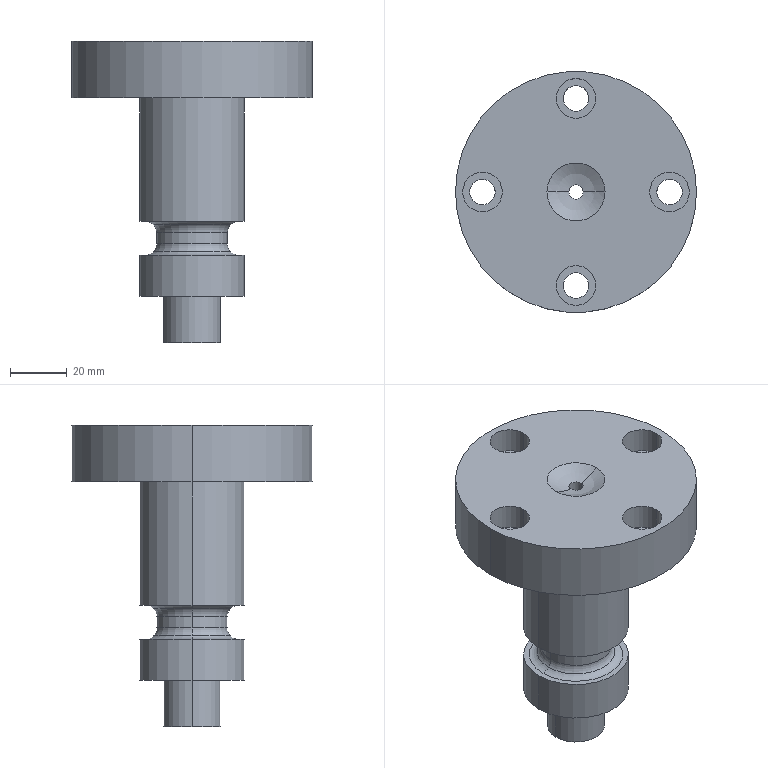Part | Creo | 1 solid | 48 faces | box 85 x 85 x 106.339 mm | volume 174751 mm3 | cylinder 26 | plane 10 | torus 8 | sphere 2 | cone 2 | commonest cylinder face diameters 9 x8 14 x8 37 x4 20 x2 25 x2 85 x2
STEP:
#1=CARTESIAN_POINT('',(18.5,0.,127.5));
#2=VERTEX_POINT('',#1);
#3=CARTESIAN_POINT('',(-18.5,0.,127.5));
#4=VERTEX_POINT('',#3);
#5=CARTESIAN_POINT('',(0.,0.,127.5));
#6=DIRECTION('',(0.,0.,1.));
#7=DIRECTION('',(1.,0.,0.));
#8=AXIS2_PLACEMENT_3D('',#5,#6,#7);
#9=CIRCLE('',#8,18.5);
#10=EDGE_CURVE('',#2,#4,#9,.T.);
#11=ORIENTED_EDGE('',*,*,#10,.T.);
#12=CARTESIAN_POINT('',(-18.5,0.,84.));
#13=VERTEX_POINT('',#12);
#14=CARTESIAN_POINT('',(-18.5,0.,127.5));
#15=DIRECTION('',(0.,0.,-1.));
#16=VECTOR('',#15,43.5);
#17=LINE('',#14,#16);
#18=EDGE_CURVE('',#4,#13,#17,.T.);
#19=ORIENTED_EDGE('',*,*,#18,.T.);
#20=CARTESIAN_POINT('',(18.5,0.,84.));
#21=VERTEX_POINT('',#20);
#22=CARTESIAN_POINT('',(0.,0.,84.));
#23=DIRECTION('',(0.,0.,-1.));
#24=DIRECTION('',(-1.,0.,0.));
#25=AXIS2_PLACEMENT_3D('',#22,#23,#24);
#26=CIRCLE('',#25,18.5);
#27=EDGE_CURVE('',#13,#21,#26,.T.);
#28=ORIENTED_EDGE('',*,*,#27,.T.);
#29=CARTESIAN_POINT('',(18.5,0.,127.5));
#30=DIRECTION('',(0.,0.,-1.));
#31=VECTOR('',#30,43.5);
#32=LINE('',#29,#31);
#33=EDGE_CURVE('',#2,#21,#32,.T.);
#34=ORIENTED_EDGE('',*,*,#33,.F.);
#35=EDGE_LOOP('',(#11,#19,#28,#34));
#36=FACE_OUTER_BOUND('',#35,.F.);
#37=CARTESIAN_POINT('',(0.,0.,127.5));
#38=DIRECTION('',(0.,0.,-1.));
#39=DIRECTION('',(-1.,0.,0.));
#40=AXIS2_PLACEMENT_3D('',#37,#38,#39);
#41=CYLINDRICAL_SURFACE('',#40,18.5);
#42=ADVANCED_FACE('',(#36),#41,.T.);
#43=CARTESIAN_POINT('',(42.5,0.,127.5));
#44=VERTEX_POINT('',#43);
#45=CARTESIAN_POINT('',(-42.5,0.,127.5));
#46=VERTEX_POINT('',#45);
#47=CARTESIAN_POINT('',(0.,0.,127.5));
#48=DIRECTION('',(0.,0.,-1.));
#49=DIRECTION('',(1.,0.,0.));
#50=AXIS2_PLACEMENT_3D('',#47,#48,#49);
#51=CIRCLE('',#50,42.5);
#52=EDGE_CURVE('',#44,#46,#51,.T.);
#53=ORIENTED_EDGE('',*,*,#52,.F.);
#54=CARTESIAN_POINT('',(0.,0.,127.5));
#55=DIRECTION('',(0.,0.,-1.));
#56=DIRECTION('',(-1.,0.,0.));
#57=AXIS2_PLACEMENT_3D('',#54,#55,#56);
#58=CIRCLE('',#57,42.5);
#59=EDGE_CURVE('',#46,#44,#58,.T.);
#60=ORIENTED_EDGE('',*,*,#59,.F.);
#61=EDGE_LOOP('',(#53,#60));
#62=FACE_OUTER_BOUND('',#61,.F.);
#63=CARTESIAN_POINT('',(-28.5,0.,127.5));
#64=VERTEX_POINT('',#63);
#65=CARTESIAN_POINT('',(-37.5,0.,127.5));
#66=VERTEX_POINT('',#65);
#67=CARTESIAN_POINT('',(-33.,0.,127.5));
#68=DIRECTION('',(0.,0.,1.));
#69=DIRECTION('',(1.,0.,0.));
#70=AXIS2_PLACEMENT_3D('',#67,#68,#69);
#71=CIRCLE('',#70,4.5);
#72=EDGE_CURVE('',#64,#66,#71,.T.);
#73=ORIENTED_EDGE('',*,*,#72,.F.);
#74=CARTESIAN_POINT('',(-33.,0.,127.5));
#75=DIRECTION('',(0.,0.,1.));
#76=DIRECTION('',(-1.,0.,0.));
#77=AXIS2_PLACEMENT_3D('',#74,#75,#76);
#78=CIRCLE('',#77,4.5);
#79=EDGE_CURVE('',#66,#64,#78,.T.);
#80=ORIENTED_EDGE('',*,*,#79,.F.);
#81=EDGE_LOOP('',(#73,#80));
#82=FACE_BOUND('',#81,.F.);
#83=CARTESIAN_POINT('',(0.,0.,127.5));
#84=DIRECTION('',(0.,0.,1.));
#85=DIRECTION('',(-1.,0.,0.));
#86=AXIS2_PLACEMENT_3D('',#83,#84,#85);
#87=CIRCLE('',#86,18.5);
#88=EDGE_CURVE('',#4,#2,#87,.T.);
#89=ORIENTED_EDGE('',*,*,#88,.F.);
#90=ORIENTED_EDGE('',*,*,#10,.F.);
#91=EDGE_LOOP('',(#89,#90));
#92=FACE_BOUND('',#91,.F.);
#93=CARTESIAN_POINT('',(4.5,33.,127.5));
#94=VERTEX_POINT('',#93);
#95=CARTESIAN_POINT('',(-4.5,33.,127.5));
#96=VERTEX_POINT('',#95);
#97=CARTESIAN_POINT('',(0.,33.,127.5));
#98=DIRECTION('',(0.,0.,1.));
#99=DIRECTION('',(1.,0.,0.));
#100=AXIS2_PLACEMENT_3D('',#97,#98,#99);
#101=CIRCLE('',#100,4.5);
#102=EDGE_CURVE('',#94,#96,#101,.T.);
#103=ORIENTED_EDGE('',*,*,#102,.F.);
#104=CARTESIAN_POINT('',(0.,33.,127.5));
#105=DIRECTION('',(0.,0.,1.));
#106=DIRECTION('',(-1.,0.,0.));
#107=AXIS2_PLACEMENT_3D('',#104,#105,#106);
#108=CIRCLE('',#107,4.5);
#109=EDGE_CURVE('',#96,#94,#108,.T.);
#110=ORIENTED_EDGE('',*,*,#109,.F.);
#111=EDGE_LOOP('',(#103,#110));
#112=FACE_BOUND('',#111,.F.);
#113=CARTESIAN_POINT('',(4.5,-33.,127.5));
#114=VERTEX_POINT('',#113);
#115=CARTESIAN_POINT('',(-4.5,-33.,127.5));
#116=VERTEX_POINT('',#115);
#117=CARTESIAN_POINT('',(0.,-33.,127.5));
#118=DIRECTION('',(0.,0.,1.));
#119=DIRECTION('',(1.,0.,0.));
#120=AXIS2_PLACEMENT_3D('',#117,#118,#119);
#121=CIRCLE('',#120,4.5);
#122=EDGE_CURVE('',#114,#116,#121,.T.);
#123=ORIENTED_EDGE('',*,*,#122,.F.);
#124=CARTESIAN_POINT('',(0.,-33.,127.5));
#125=DIRECTION('',(0.,0.,1.));
#126=DIRECTION('',(-1.,0.,0.));
#127=AXIS2_PLACEMENT_3D('',#124,#125,#126);
#128=CIRCLE('',#127,4.5);
#129=EDGE_CURVE('',#116,#114,#128,.T.);
#130=ORIENTED_EDGE('',*,*,#129,.F.);
#131=EDGE_LOOP('',(#123,#130));
#132=FACE_BOUND('',#131,.F.);
#133=CARTESIAN_POINT('',(37.5,0.,127.5));
#134=VERTEX_POINT('',#133);
#135=CARTESIAN_POINT('',(28.5,0.,127.5));
#136=VERTEX_POINT('',#135);
#137=CARTESIAN_POINT('',(33.,0.,127.5));
#138=DIRECTION('',(0.,0.,1.));
#139=DIRECTION('',(1.,0.,0.));
#140=AXIS2_PLACEMENT_3D('',#137,#138,#139);
#141=CIRCLE('',#140,4.5);
#142=EDGE_CURVE('',#134,#136,#141,.T.);
#143=ORIENTED_EDGE('',*,*,#142,.F.);
#144=CARTESIAN_POINT('',(33.,0.,127.5));
#145=DIRECTION('',(0.,0.,1.));
#146=DIRECTION('',(-1.,0.,0.));
#147=AXIS2_PLACEMENT_3D('',#144,#145,#146);
#148=CIRCLE('',#147,4.5);
#149=EDGE_CURVE('',#136,#134,#148,.T.);
#150=ORIENTED_EDGE('',*,*,#149,.F.);
#151=EDGE_LOOP('',(#143,#150));
#152=FACE_BOUND('',#151,.F.);
#153=CARTESIAN_POINT('',(0.,0.,127.5));
#154=DIRECTION('',(0.,0.,-1.));
#155=DIRECTION('',(-1.,0.,0.));
#156=AXIS2_PLACEMENT_3D('',#153,#154,#155);
#157=PLANE('',#156);
#158=ADVANCED_FACE('',(#62,#82,#92,#112,#132,#152),#157,.T.);
#159=CARTESIAN_POINT('',(-4.5,33.,138.5));
#160=VERTEX_POINT('',#159);
#161=CARTESIAN_POINT('',(4.5,33.,138.5));
#162=VERTEX_POINT('',#161);
#163=CARTESIAN_POINT('',(0.,33.,138.5));
#164=DIRECTION('',(0.,0.,-1.));
#165=DIRECTION('',(-1.,0.,0.));
#166=AXIS2_PLACEMENT_3D('',#163,#164,#165);
#167=CIRCLE('',#166,4.5);
#168=EDGE_CURVE('',#160,#162,#167,.T.);
#169=ORIENTED_EDGE('',*,*,#168,.T.);
#170=CARTESIAN_POINT('',(4.5,33.,127.5));
#171=DIRECTION('',(0.,0.,1.));
#172=VECTOR('',#171,11.);
#173=LINE('',#170,#172);
#174=EDGE_CURVE('',#94,#162,#173,.T.);
#175=ORIENTED_EDGE('',*,*,#174,.F.);
#176=ORIENTED_EDGE('',*,*,#102,.T.);
#177=CARTESIAN_POINT('',(-4.5,33.,127.5));
#178=DIRECTION('',(0.,0.,1.));
#179=VECTOR('',#178,11.);
#180=LINE('',#177,#179);
#181=EDGE_CURVE('',#96,#160,#180,.T.);
#182=ORIENTED_EDGE('',*,*,#181,.T.);
#183=EDGE_LOOP('',(#169,#175,#176,#182));
#184=FACE_OUTER_BOUND('',#183,.F.);
#185=CARTESIAN_POINT('',(0.,33.,127.5));
#186=DIRECTION('',(0.,0.,1.));
#187=DIRECTION('',(1.,0.,0.));
#188=AXIS2_PLACEMENT_3D('',#185,#186,#187);
#189=CYLINDRICAL_SURFACE('',#188,4.5);
#190=ADVANCED_FACE('',(#184),#189,.F.);
#191=CARTESIAN_POINT('',(7.,33.,138.5));
#192=VERTEX_POINT('',#191);
#193=CARTESIAN_POINT('',(-7.,33.,138.5));
#194=VERTEX_POINT('',#193);
#195=CARTESIAN_POINT('',(0.,33.,138.5));
#196=DIRECTION('',(0.,0.,1.));
#197=DIRECTION('',(1.,0.,0.));
#198=AXIS2_PLACEMENT_3D('',#195,#196,#197);
#199=CIRCLE('',#198,7.);
#200=EDGE_CURVE('',#192,#194,#199,.T.);
#201=ORIENTED_EDGE('',*,*,#200,.F.);
#202=CARTESIAN_POINT('',(0.,33.,138.5));
#203=DIRECTION('',(0.,0.,1.));
#204=DIRECTION('',(-1.,0.,0.));
#205=AXIS2_PLACEMENT_3D('',#202,#203,#204);
#206=CIRCLE('',#205,7.);
#207=EDGE_CURVE('',#194,#192,#206,.T.);
#208=ORIENTED_EDGE('',*,*,#207,.F.);
#209=EDGE_LOOP('',(#201,#208));
#210=FACE_OUTER_BOUND('',#209,.F.);
#211=CARTESIAN_POINT('',(0.,33.,138.5));
#212=DIRECTION('',(0.,0.,-1.));
#213=DIRECTION('',(1.,0.,0.));
#214=AXIS2_PLACEMENT_3D('',#211,#212,#213);
#215=CIRCLE('',#214,4.5);
#216=EDGE_CURVE('',#162,#160,#215,.T.);
#217=ORIENTED_EDGE('',*,*,#216,.F.);
#218=ORIENTED_EDGE('',*,*,#168,.F.);
#219=EDGE_LOOP('',(#217,#218));
#220=FACE_BOUND('',#219,.F.);
#221=CARTESIAN_POINT('',(0.,33.,138.5));
#222=DIRECTION('',(0.,0.,-1.));
#223=DIRECTION('',(-1.,0.,0.));
#224=AXIS2_PLACEMENT_3D('',#221,#222,#223);
#225=PLANE('',#224);
#226=ADVANCED_FACE('',(#210,#220),#225,.F.);
#227=ORIENTED_EDGE('',*,*,#216,.T.);
#228=ORIENTED_EDGE('',*,*,#181,.F.);
#229=ORIENTED_EDGE('',*,*,#109,.T.);
#230=ORIENTED_EDGE('',*,*,#174,.T.);
#231=EDGE_LOOP('',(#227,#228,#229,#230));
#232=FACE_OUTER_BOUND('',#231,.F.);
#233=CARTESIAN_POINT('',(0.,33.,127.5));
#234=DIRECTION('',(0.,0.,1.));
#235=DIRECTION('',(1.,0.,0.));
#236=AXIS2_PLACEMENT_3D('',#233,#234,#235);
#237=CYLINDRICAL_SURFACE('',#236,4.5);
#238=ADVANCED_FACE('',(#232),#237,.F.);
#239=CARTESIAN_POINT('',(-7.,33.,147.5));
#240=VERTEX_POINT('',#239);
#241=CARTESIAN_POINT('',(7.,33.,147.5));
#242=VERTEX_POINT('',#241);
#243=CARTESIAN_POINT('',(0.,33.,147.5));
#244=DIRECTION('',(0.,0.,-1.));
#245=DIRECTION('',(-1.,0.,0.));
#246=AXIS2_PLACEMENT_3D('',#243,#244,#245);
#247=CIRCLE('',#246,7.);
#248=EDGE_CURVE('',#240,#242,#247,.T.);
#249=ORIENTED_EDGE('',*,*,#248,.T.);
#250=CARTESIAN_POINT('',(7.,33.,138.5));
#251=DIRECTION('',(0.,0.,1.));
#252=VECTOR('',#251,9.);
#253=LINE('',#250,#252);
#254=EDGE_CURVE('',#192,#242,#253,.T.);
#255=ORIENTED_EDGE('',*,*,#254,.F.);
#256=ORIENTED_EDGE('',*,*,#200,.T.);
#257=CARTESIAN_POINT('',(-7.,33.,138.5));
#258=DIRECTION('',(0.,0.,1.));
#259=VECTOR('',#258,9.);
#260=LINE('',#257,#259);
#261=EDGE_CURVE('',#194,#240,#260,.T.);
#262=ORIENTED_EDGE('',*,*,#261,.T.);
#263=EDGE_LOOP('',(#249,#255,#256,#262));
#264=FACE_OUTER_BOUND('',#263,.F.);
#265=CARTESIAN_POINT('',(0.,33.,138.5));
#266=DIRECTION('',(0.,0.,1.));
#267=DIRECTION('',(1.,0.,0.));
#268=AXIS2_PLACEMENT_3D('',#265,#266,#267);
#269=CYLINDRICAL_SURFACE('',#268,7.);
#270=ADVANCED_FACE('',(#264),#269,.F.);
#271=CARTESIAN_POINT('',(-42.5,0.,147.5));
#272=VERTEX_POINT('',#271);
#273=CARTESIAN_POINT('',(42.5,0.,147.5));
#274=VERTEX_POINT('',#273);
#275=CARTESIAN_POINT('',(0.,0.,147.5));
#276=DIRECTION('',(0.,0.,1.));
#277=DIRECTION('',(-1.,0.,0.));
#278=AXIS2_PLACEMENT_3D('',#275,#276,#277);
#279=CIRCLE('',#278,42.5);
#280=EDGE_CURVE('',#272,#274,#279,.T.);
#281=ORIENTED_EDGE('',*,*,#280,.F.);
#282=CARTESIAN_POINT('',(0.,0.,147.5));
#283=DIRECTION('',(0.,0.,1.));
#284=DIRECTION('',(1.,0.,0.));
#285=AXIS2_PLACEMENT_3D('',#282,#283,#284);
#286=CIRCLE('',#285,42.5);
#287=EDGE_CURVE('',#274,#272,#286,.T.);
#288=ORIENTED_EDGE('',*,*,#287,.F.);
#289=EDGE_LOOP('',(#281,#288));
#290=FACE_OUTER_BOUND('',#289,.F.);
#291=CARTESIAN_POINT('',(0.,33.,147.5));
#292=DIRECTION('',(0.,0.,-1.));
#293=DIRECTION('',(1.,0.,0.));
#294=AXIS2_PLACEMENT_3D('',#291,#292,#293);
#295=CIRCLE('',#294,7.);
#296=EDGE_CURVE('',#242,#240,#295,.T.);
#297=ORIENTED_EDGE('',*,*,#296,.F.);
#298=ORIENTED_EDGE('',*,*,#248,.F.);
#299=EDGE_LOOP('',(#297,#298));
#300=FACE_BOUND('',#299,.F.);
#301=CARTESIAN_POINT('',(7.,-33.,147.5));
#302=VERTEX_POINT('',#301);
#303=CARTESIAN_POINT('',(-7.,-33.,147.5));
#304=VERTEX_POINT('',#303);
#305=CARTESIAN_POINT('',(0.,-33.,147.5));
#306=DIRECTION('',(0.,0.,-1.));
#307=DIRECTION('',(1.,0.,0.));
#308=AXIS2_PLACEMENT_3D('',#305,#306,#307);
#309=CIRCLE('',#308,7.);
#310=EDGE_CURVE('',#302,#304,#309,.T.);
#311=ORIENTED_EDGE('',*,*,#310,.F.);
#312=CARTESIAN_POINT('',(0.,-33.,147.5));
#313=DIRECTION('',(0.,0.,-1.));
#314=DIRECTION('',(-1.,0.,0.));
#315=AXIS2_PLACEMENT_3D('',#312,#313,#314);
#316=CIRCLE('',#315,7.);
#317=EDGE_CURVE('',#304,#302,#316,.T.);
#318=ORIENTED_EDGE('',*,*,#317,.F.);
#319=EDGE_LOOP('',(#311,#318));
#320=FACE_BOUND('',#319,.F.);
#321=CARTESIAN_POINT('',(-26.,0.,147.5));
#322=VERTEX_POINT('',#321);
#323=CARTESIAN_POINT('',(-40.,0.,147.5));
#324=VERTEX_POINT('',#323);
#325=CARTESIAN_POINT('',(-33.,0.,147.5));
#326=DIRECTION('',(0.,0.,-1.));
#327=DIRECTION('',(1.,0.,0.));
#328=AXIS2_PLACEMENT_3D('',#325,#326,#327);
#329=CIRCLE('',#328,7.);
#330=EDGE_CURVE('',#322,#324,#329,.T.);
#331=ORIENTED_EDGE('',*,*,#330,.F.);
#332=CARTESIAN_POINT('',(-33.,0.,147.5));
#333=DIRECTION('',(0.,0.,-1.));
#334=DIRECTION('',(-1.,0.,0.));
#335=AXIS2_PLACEMENT_3D('',#332,#333,#334);
#336=CIRCLE('',#335,7.);
#337=EDGE_CURVE('',#324,#322,#336,.T.);
#338=ORIENTED_EDGE('',*,*,#337,.F.);
#339=EDGE_LOOP('',(#331,#338));
#340=FACE_BOUND('',#339,.F.);
#341=CARTESIAN_POINT('',(10.247,0.,147.5));
#342=VERTEX_POINT('',#341);
#343=CARTESIAN_POINT('',(-10.247,0.,147.5));
#344=VERTEX_POINT('',#343);
#345=CARTESIAN_POINT('',(0.,0.,147.5));
#346=DIRECTION('',(0.,0.,-1.));
#347=DIRECTION('',(1.,0.,0.));
#348=AXIS2_PLACEMENT_3D('',#345,#346,#347);
#349=CIRCLE('',#348,10.247);
#350=EDGE_CURVE('',#342,#344,#349,.T.);
#351=ORIENTED_EDGE('',*,*,#350,.F.);
#352=CARTESIAN_POINT('',(0.,0.,147.5));
#353=DIRECTION('',(0.,0.,-1.));
#354=DIRECTION('',(-1.,0.,0.));
#355=AXIS2_PLACEMENT_3D('',#352,#353,#354);
#356=CIRCLE('',#355,10.247);
#357=EDGE_CURVE('',#344,#342,#356,.T.);
#358=ORIENTED_EDGE('',*,*,#357,.F.);
#359=EDGE_LOOP('',(#351,#358));
#360=FACE_BOUND('',#359,.F.);
#361=CARTESIAN_POINT('',(40.,0.,147.5));
#362=VERTEX_POINT('',#361);
#363=CARTESIAN_POINT('',(26.,0.,147.5));
#364=VERTEX_POINT('',#363);
#365=CARTESIAN_POINT('',(33.,0.,147.5));
#366=DIRECTION('',(0.,0.,-1.));
#367=DIRECTION('',(1.,0.,0.));
#368=AXIS2_PLACEMENT_3D('',#365,#366,#367);
#369=CIRCLE('',#368,7.);
#370=EDGE_CURVE('',#362,#364,#369,.T.);
#371=ORIENTED_EDGE('',*,*,#370,.F.);
#372=CARTESIAN_POINT('',(33.,0.,147.5));
#373=DIRECTION('',(0.,0.,-1.));
#374=DIRECTION('',(-1.,0.,0.));
#375=AXIS2_PLACEMENT_3D('',#372,#373,#374);
#376=CIRCLE('',#375,7.);
#377=EDGE_CURVE('',#364,#362,#376,.T.);
#378=ORIENTED_EDGE('',*,*,#377,.F.);
#379=EDGE_LOOP('',(#371,#378));
#380=FACE_BOUND('',#379,.F.);
#381=CARTESIAN_POINT('',(0.,0.,147.5));
#382=DIRECTION('',(0.,0.,1.));
#383=DIRECTION('',(1.,0.,0.));
#384=AXIS2_PLACEMENT_3D('',#381,#382,#383);
#385=PLANE('',#384);
#386=ADVANCED_FACE('',(#290,#300,#320,#340,#360,#380),#385,.T.);
#387=ORIENTED_EDGE('',*,*,#370,.T.);
#388=CARTESIAN_POINT('',(26.,0.,138.5));
#389=VERTEX_POINT('',#388);
#390=CARTESIAN_POINT('',(26.,0.,138.5));
#391=DIRECTION('',(0.,0.,1.));
#392=VECTOR('',#391,9.);
#393=LINE('',#390,#392);
#394=EDGE_CURVE('',#389,#364,#393,.T.);
#395=ORIENTED_EDGE('',*,*,#394,.F.);
#396=CARTESIAN_POINT('',(40.,0.,138.5));
#397=VERTEX_POINT('',#396);
#398=CARTESIAN_POINT('',(33.,0.,138.5));
#399=DIRECTION('',(0.,0.,1.));
#400=DIRECTION('',(-1.,0.,0.));
#401=AXIS2_PLACEMENT_3D('',#398,#399,#400);
#402=CIRCLE('',#401,7.);
#403=EDGE_CURVE('',#389,#397,#402,.T.);
#404=ORIENTED_EDGE('',*,*,#403,.T.);
#405=CARTESIAN_POINT('',(40.,0.,138.5));
#406=DIRECTION('',(0.,0.,1.));
#407=VECTOR('',#406,9.);
#408=LINE('',#405,#407);
#409=EDGE_CURVE('',#397,#362,#408,.T.);
#410=ORIENTED_EDGE('',*,*,#409,.T.);
#411=EDGE_LOOP('',(#387,#395,#404,#410));
#412=FACE_OUTER_BOUND('',#411,.F.);
#413=CARTESIAN_POINT('',(33.,0.,138.5));
#414=DIRECTION('',(0.,0.,1.));
#415=DIRECTION('',(1.,0.,0.));
#416=AXIS2_PLACEMENT_3D('',#413,#414,#415);
#417=CYLINDRICAL_SURFACE('',#416,7.);
#418=ADVANCED_FACE('',(#412),#417,.F.);
#419=ORIENTED_EDGE('',*,*,#377,.T.);
#420=ORIENTED_EDGE('',*,*,#409,.F.);
#421=CARTESIAN_POINT('',(33.,0.,138.5));
#422=DIRECTION('',(0.,0.,1.));
#423=DIRECTION('',(1.,0.,0.));
#424=AXIS2_PLACEMENT_3D('',#421,#422,#423);
#425=CIRCLE('',#424,7.);
#426=EDGE_CURVE('',#397,#389,#425,.T.);
#427=ORIENTED_EDGE('',*,*,#426,.T.);
#428=ORIENTED_EDGE('',*,*,#394,.T.);
#429=EDGE_LOOP('',(#419,#420,#427,#428));
#430=FACE_OUTER_BOUND('',#429,.F.);
#431=CARTESIAN_POINT('',(33.,0.,138.5));
#432=DIRECTION('',(0.,0.,1.));
#433=DIRECTION('',(1.,0.,0.));
#434=AXIS2_PLACEMENT_3D('',#431,#432,#433);
#435=CYLINDRICAL_SURFACE('',#434,7.);
#436=ADVANCED_FACE('',(#430),#435,.F.);
#437=ORIENTED_EDGE('',*,*,#426,.F.);
#438=ORIENTED_EDGE('',*,*,#403,.F.);
#439=EDGE_LOOP('',(#437,#438));
#440=FACE_OUTER_BOUND('',#439,.F.);
#441=CARTESIAN_POINT('',(37.5,0.,138.5));
#442=VERTEX_POINT('',#441);
#443=CARTESIAN_POINT('',(28.5,0.,138.5));
#444=VERTEX_POINT('',#443);
#445=CARTESIAN_POINT('',(33.,0.,138.5));
#446=DIRECTION('',(0.,0.,-1.));
#447=DIRECTION('',(1.,0.,0.));
#448=AXIS2_PLACEMENT_3D('',#445,#446,#447);
#449=CIRCLE('',#448,4.5);
#450=EDGE_CURVE('',#442,#444,#449,.T.);
#451=ORIENTED_EDGE('',*,*,#450,.F.);
#452=CARTESIAN_POINT('',(33.,0.,138.5));
#453=DIRECTION('',(0.,0.,-1.));
#454=DIRECTION('',(-1.,0.,0.));
#455=AXIS2_PLACEMENT_3D('',#452,#453,#454);
#456=CIRCLE('',#455,4.5);
#457=EDGE_CURVE('',#444,#442,#456,.T.);
#458=ORIENTED_EDGE('',*,*,#457,.F.);
#459=EDGE_LOOP('',(#451,#458));
#460=FACE_BOUND('',#459,.F.);
#461=CARTESIAN_POINT('',(33.,0.,138.5));
#462=DIRECTION('',(0.,0.,-1.));
#463=DIRECTION('',(-1.,0.,0.));
#464=AXIS2_PLACEMENT_3D('',#461,#462,#463);
#465=PLANE('',#464);
#466=ADVANCED_FACE('',(#440,#460),#465,.F.);
#467=ORIENTED_EDGE('',*,*,#450,.T.);
#468=CARTESIAN_POINT('',(28.5,0.,127.5));
#469=DIRECTION('',(0.,0.,1.));
#470=VECTOR('',#469,11.);
#471=LINE('',#468,#470);
#472=EDGE_CURVE('',#136,#444,#471,.T.);
#473=ORIENTED_EDGE('',*,*,#472,.F.);
#474=ORIENTED_EDGE('',*,*,#149,.T.);
#475=CARTESIAN_POINT('',(37.5,0.,127.5));
#476=DIRECTION('',(0.,0.,1.));
#477=VECTOR('',#476,11.);
#478=LINE('',#475,#477);
#479=EDGE_CURVE('',#134,#442,#478,.T.);
#480=ORIENTED_EDGE('',*,*,#479,.T.);
#481=EDGE_LOOP('',(#467,#473,#474,#480));
#482=FACE_OUTER_BOUND('',#481,.F.);
#483=CARTESIAN_POINT('',(33.,0.,127.5));
#484=DIRECTION('',(0.,0.,1.));
#485=DIRECTION('',(1.,0.,0.));
#486=AXIS2_PLACEMENT_3D('',#483,#484,#485);
#487=CYLINDRICAL_SURFACE('',#486,4.5);
#488=ADVANCED_FACE('',(#482),#487,.F.);
#489=ORIENTED_EDGE('',*,*,#457,.T.);
#490=ORIENTED_EDGE('',*,*,#479,.F.);
#491=ORIENTED_EDGE('',*,*,#142,.T.);
#492=ORIENTED_EDGE('',*,*,#472,.T.);
#493=EDGE_LOOP('',(#489,#490,#491,#492));
#494=FACE_OUTER_BOUND('',#493,.F.);
#495=CARTESIAN_POINT('',(33.,0.,127.5));
#496=DIRECTION('',(0.,0.,1.));
#497=DIRECTION('',(1.,0.,0.));
#498=AXIS2_PLACEMENT_3D('',#495,#496,#497);
#499=CYLINDRICAL_SURFACE('',#498,4.5);
#500=ADVANCED_FACE('',(#494),#499,.F.);
#501=ORIENTED_EDGE('',*,*,#296,.T.);
#502=ORIENTED_EDGE('',*,*,#261,.F.);
#503=ORIENTED_EDGE('',*,*,#207,.T.);
#504=ORIENTED_EDGE('',*,*,#254,.T.);
#505=EDGE_LOOP('',(#501,#502,#503,#504));
#506=FACE_OUTER_BOUND('',#505,.F.);
#507=CARTESIAN_POINT('',(0.,33.,138.5));
#508=DIRECTION('',(0.,0.,1.));
#509=DIRECTION('',(1.,0.,0.));
#510=AXIS2_PLACEMENT_3D('',#507,#508,#509);
#511=CYLINDRICAL_SURFACE('',#510,7.);
#512=ADVANCED_FACE('',(#506),#511,.F.);
#513=ORIENTED_EDGE('',*,*,#310,.T.);
#514=CARTESIAN_POINT('',(-7.,-33.,138.5));
#515=VERTEX_POINT('',#514);
#516=CARTESIAN_POINT('',(-7.,-33.,138.5));
#517=DIRECTION('',(0.,0.,1.));
#518=VECTOR('',#517,9.);
#519=LINE('',#516,#518);
#520=EDGE_CURVE('',#515,#304,#519,.T.);
#521=ORIENTED_EDGE('',*,*,#520,.F.);
#522=CARTESIAN_POINT('',(7.,-33.,138.5));
#523=VERTEX_POINT('',#522);
#524=CARTESIAN_POINT('',(0.,-33.,138.5));
#525=DIRECTION('',(0.,0.,1.));
#526=DIRECTION('',(-1.,0.,0.));
#527=AXIS2_PLACEMENT_3D('',#524,#525,#526);
#528=CIRCLE('',#527,7.);
#529=EDGE_CURVE('',#515,#523,#528,.T.);
#530=ORIENTED_EDGE('',*,*,#529,.T.);
#531=CARTESIAN_POINT('',(7.,-33.,138.5));
#532=DIRECTION('',(0.,0.,1.));
#533=VECTOR('',#532,9.);
#534=LINE('',#531,#533);
#535=EDGE_CURVE('',#523,#302,#534,.T.);
#536=ORIENTED_EDGE('',*,*,#535,.T.);
#537=EDGE_LOOP('',(#513,#521,#530,#536));
#538=FACE_OUTER_BOUND('',#537,.F.);
#539=CARTESIAN_POINT('',(0.,-33.,138.5));
#540=DIRECTION('',(0.,0.,1.));
#541=DIRECTION('',(1.,0.,0.));
#542=AXIS2_PLACEMENT_3D('',#539,#540,#541);
#543=CYLINDRICAL_SURFACE('',#542,7.);
#544=ADVANCED_FACE('',(#538),#543,.F.);
#545=ORIENTED_EDGE('',*,*,#317,.T.);
#546=ORIENTED_EDGE('',*,*,#535,.F.);
#547=CARTESIAN_POINT('',(0.,-33.,138.5));
#548=DIRECTION('',(0.,0.,1.));
#549=DIRECTION('',(1.,0.,0.));
#550=AXIS2_PLACEMENT_3D('',#547,#548,#549);
#551=CIRCLE('',#550,7.);
#552=EDGE_CURVE('',#523,#515,#551,.T.);
#553=ORIENTED_EDGE('',*,*,#552,.T.);
#554=ORIENTED_EDGE('',*,*,#520,.T.);
#555=EDGE_LOOP('',(#545,#546,#553,#554));
#556=FACE_OUTER_BOUND('',#555,.F.);
#557=CARTESIAN_POINT('',(0.,-33.,138.5));
#558=DIRECTION('',(0.,0.,1.));
#559=DIRECTION('',(1.,0.,0.));
#560=AXIS2_PLACEMENT_3D('',#557,#558,#559);
#561=CYLINDRICAL_SURFACE('',#560,7.);
#562=ADVANCED_FACE('',(#556),#561,.F.);
#563=ORIENTED_EDGE('',*,*,#552,.F.);
#564=ORIENTED_EDGE('',*,*,#529,.F.);
#565=EDGE_LOOP('',(#563,#564));
#566=FACE_OUTER_BOUND('',#565,.F.);
#567=CARTESIAN_POINT('',(4.5,-33.,138.5));
#568=VERTEX_POINT('',#567);
#569=CARTESIAN_POINT('',(-4.5,-33.,138.5));
#570=VERTEX_POINT('',#569);
#571=CARTESIAN_POINT('',(0.,-33.,138.5));
#572=DIRECTION('',(0.,0.,-1.));
#573=DIRECTION('',(1.,0.,0.));
#574=AXIS2_PLACEMENT_3D('',#571,#572,#573);
#575=CIRCLE('',#574,4.5);
#576=EDGE_CURVE('',#568,#570,#575,.T.);
#577=ORIENTED_EDGE('',*,*,#576,.F.);
#578=CARTESIAN_POINT('',(0.,-33.,138.5));
#579=DIRECTION('',(0.,0.,-1.));
#580=DIRECTION('',(-1.,0.,0.));
#581=AXIS2_PLACEMENT_3D('',#578,#579,#580);
#582=CIRCLE('',#581,4.5);
#583=EDGE_CURVE('',#570,#568,#582,.T.);
#584=ORIENTED_EDGE('',*,*,#583,.F.);
#585=EDGE_LOOP('',(#577,#584));
#586=FACE_BOUND('',#585,.F.);
#587=CARTESIAN_POINT('',(0.,-33.,138.5));
#588=DIRECTION('',(0.,0.,-1.));
#589=DIRECTION('',(-1.,0.,0.));
#590=AXIS2_PLACEMENT_3D('',#587,#588,#589);
#591=PLANE('',#590);
#592=ADVANCED_FACE('',(#566,#586),#591,.F.);
#593=ORIENTED_EDGE('',*,*,#576,.T.);
#594=CARTESIAN_POINT('',(-4.5,-33.,127.5));
#595=DIRECTION('',(0.,0.,1.));
#596=VECTOR('',#595,11.);
#597=LINE('',#594,#596);
#598=EDGE_CURVE('',#116,#570,#597,.T.);
#599=ORIENTED_EDGE('',*,*,#598,.F.);
#600=ORIENTED_EDGE('',*,*,#129,.T.);
#601=CARTESIAN_POINT('',(4.5,-33.,127.5));
#602=DIRECTION('',(0.,0.,1.));
#603=VECTOR('',#602,11.);
#604=LINE('',#601,#603);
#605=EDGE_CURVE('',#114,#568,#604,.T.);
#606=ORIENTED_EDGE('',*,*,#605,.T.);
#607=EDGE_LOOP('',(#593,#599,#600,#606));
#608=FACE_OUTER_BOUND('',#607,.F.);
#609=CARTESIAN_POINT('',(0.,-33.,127.5));
#610=DIRECTION('',(0.,0.,1.));
#611=DIRECTION('',(1.,0.,0.));
#612=AXIS2_PLACEMENT_3D('',#609,#610,#611);
#613=CYLINDRICAL_SURFACE('',#612,4.5);
#614=ADVANCED_FACE('',(#608),#613,.F.);
#615=ORIENTED_EDGE('',*,*,#583,.T.);
#616=ORIENTED_EDGE('',*,*,#605,.F.);
#617=ORIENTED_EDGE('',*,*,#122,.T.);
#618=ORIENTED_EDGE('',*,*,#598,.T.);
#619=EDGE_LOOP('',(#615,#616,#617,#618));
#620=FACE_OUTER_BOUND('',#619,.F.);
#621=CARTESIAN_POINT('',(0.,-33.,127.5));
#622=DIRECTION('',(0.,0.,1.));
#623=DIRECTION('',(1.,0.,0.));
#624=AXIS2_PLACEMENT_3D('',#621,#622,#623);
#625=CYLINDRICAL_SURFACE('',#624,4.5);
#626=ADVANCED_FACE('',(#620),#625,.F.);
#627=ORIENTED_EDGE('',*,*,#330,.T.);
#628=CARTESIAN_POINT('',(-40.,0.,138.5));
#629=VERTEX_POINT('',#628);
#630=CARTESIAN_POINT('',(-40.,0.,138.5));
#631=DIRECTION('',(0.,0.,1.));
#632=VECTOR('',#631,9.);
#633=LINE('',#630,#632);
#634=EDGE_CURVE('',#629,#324,#633,.T.);
#635=ORIENTED_EDGE('',*,*,#634,.F.);
#636=CARTESIAN_POINT('',(-26.,0.,138.5));
#637=VERTEX_POINT('',#636);
#638=CARTESIAN_POINT('',(-33.,0.,138.5));
#639=DIRECTION('',(0.,0.,1.));
#640=DIRECTION('',(-1.,0.,0.));
#641=AXIS2_PLACEMENT_3D('',#638,#639,#640);
#642=CIRCLE('',#641,7.);
#643=EDGE_CURVE('',#629,#637,#642,.T.);
#644=ORIENTED_EDGE('',*,*,#643,.T.);
#645=CARTESIAN_POINT('',(-26.,0.,138.5));
#646=DIRECTION('',(0.,0.,1.));
#647=VECTOR('',#646,9.);
#648=LINE('',#645,#647);
#649=EDGE_CURVE('',#637,#322,#648,.T.);
#650=ORIENTED_EDGE('',*,*,#649,.T.);
#651=EDGE_LOOP('',(#627,#635,#644,#650));
#652=FACE_OUTER_BOUND('',#651,.F.);
#653=CARTESIAN_POINT('',(-33.,0.,138.5));
#654=DIRECTION('',(0.,0.,1.));
#655=DIRECTION('',(1.,0.,0.));
#656=AXIS2_PLACEMENT_3D('',#653,#654,#655);
#657=CYLINDRICAL_SURFACE('',#656,7.);
#658=ADVANCED_FACE('',(#652),#657,.F.);
#659=ORIENTED_EDGE('',*,*,#337,.T.);
#660=ORIENTED_EDGE('',*,*,#649,.F.);
#661=CARTESIAN_POINT('',(-33.,0.,138.5));
#662=DIRECTION('',(0.,0.,1.));
#663=DIRECTION('',(1.,0.,0.));
#664=AXIS2_PLACEMENT_3D('',#661,#662,#663);
#665=CIRCLE('',#664,7.);
#666=EDGE_CURVE('',#637,#629,#665,.T.);
#667=ORIENTED_EDGE('',*,*,#666,.T.);
#668=ORIENTED_EDGE('',*,*,#634,.T.);
#669=EDGE_LOOP('',(#659,#660,#667,#668));
#670=FACE_OUTER_BOUND('',#669,.F.);
#671=CARTESIAN_POINT('',(-33.,0.,138.5));
#672=DIRECTION('',(0.,0.,1.));
#673=DIRECTION('',(1.,0.,0.));
#674=AXIS2_PLACEMENT_3D('',#671,#672,#673);
#675=CYLINDRICAL_SURFACE('',#674,7.);
#676=ADVANCED_FACE('',(#670),#675,.F.);
#677=ORIENTED_EDGE('',*,*,#666,.F.);
#678=ORIENTED_EDGE('',*,*,#643,.F.);
#679=EDGE_LOOP('',(#677,#678));
#680=FACE_OUTER_BOUND('',#679,.F.);
#681=CARTESIAN_POINT('',(-28.5,0.,138.5));
#682=VERTEX_POINT('',#681);
#683=CARTESIAN_POINT('',(-37.5,0.,138.5));
#684=VERTEX_POINT('',#683);
#685=CARTESIAN_POINT('',(-33.,0.,138.5));
#686=DIRECTION('',(0.,0.,-1.));
#687=DIRECTION('',(1.,0.,0.));
#688=AXIS2_PLACEMENT_3D('',#685,#686,#687);
#689=CIRCLE('',#688,4.5);
#690=EDGE_CURVE('',#682,#684,#689,.T.);
#691=ORIENTED_EDGE('',*,*,#690,.F.);
#692=CARTESIAN_POINT('',(-33.,0.,138.5));
#693=DIRECTION('',(0.,0.,-1.));
#694=DIRECTION('',(-1.,0.,0.));
#695=AXIS2_PLACEMENT_3D('',#692,#693,#694);
#696=CIRCLE('',#695,4.5);
#697=EDGE_CURVE('',#684,#682,#696,.T.);
#698=ORIENTED_EDGE('',*,*,#697,.F.);
#699=EDGE_LOOP('',(#691,#698));
#700=FACE_BOUND('',#699,.F.);
#701=CARTESIAN_POINT('',(-33.,0.,138.5));
#702=DIRECTION('',(0.,0.,-1.));
#703=DIRECTION('',(-1.,0.,0.));
#704=AXIS2_PLACEMENT_3D('',#701,#702,#703);
#705=PLANE('',#704);
#706=ADVANCED_FACE('',(#680,#700),#705,.F.);
#707=ORIENTED_EDGE('',*,*,#690,.T.);
#708=CARTESIAN_POINT('',(-37.5,0.,127.5));
#709=DIRECTION('',(0.,0.,1.));
#710=VECTOR('',#709,11.);
#711=LINE('',#708,#710);
#712=EDGE_CURVE('',#66,#684,#711,.T.);
#713=ORIENTED_EDGE('',*,*,#712,.F.);
#714=ORIENTED_EDGE('',*,*,#79,.T.);
#715=CARTESIAN_POINT('',(-28.5,0.,127.5));
#716=DIRECTION('',(0.,0.,1.));
#717=VECTOR('',#716,11.);
#718=LINE('',#715,#717);
#719=EDGE_CURVE('',#64,#682,#718,.T.);
#720=ORIENTED_EDGE('',*,*,#719,.T.);
#721=EDGE_LOOP('',(#707,#713,#714,#720));
#722=FACE_OUTER_BOUND('',#721,.F.);
#723=CARTESIAN_POINT('',(-33.,0.,127.5));
#724=DIRECTION('',(0.,0.,1.));
#725=DIRECTION('',(1.,0.,0.));
#726=AXIS2_PLACEMENT_3D('',#723,#724,#725);
#727=CYLINDRICAL_SURFACE('',#726,4.5);
#728=ADVANCED_FACE('',(#722),#727,.F.);
#729=ORIENTED_EDGE('',*,*,#697,.T.);
#730=ORIENTED_EDGE('',*,*,#719,.F.);
#731=ORIENTED_EDGE('',*,*,#72,.T.);
#732=ORIENTED_EDGE('',*,*,#712,.T.);
#733=EDGE_LOOP('',(#729,#730,#731,#732));
#734=FACE_OUTER_BOUND('',#733,.F.);
#735=CARTESIAN_POINT('',(-33.,0.,127.5));
#736=DIRECTION('',(0.,0.,1.));
#737=DIRECTION('',(1.,0.,0.));
#738=AXIS2_PLACEMENT_3D('',#735,#736,#737);
#739=CYLINDRICAL_SURFACE('',#738,4.5);
#740=ADVANCED_FACE('',(#734),#739,.F.);
#741=CARTESIAN_POINT('',(2.5,0.,144.665));
#742=VERTEX_POINT('',#741);
#743=CARTESIAN_POINT('',(-2.5,0.,144.665));
#744=VERTEX_POINT('',#743);
#745=CARTESIAN_POINT('',(0.,0.,144.665));
#746=DIRECTION('',(0.,0.,-1.));
#747=DIRECTION('',(1.,0.,0.));
#748=AXIS2_PLACEMENT_3D('',#745,#746,#747);
#749=CIRCLE('',#748,2.5);
#750=EDGE_CURVE('',#742,#744,#749,.T.);
#751=ORIENTED_EDGE('',*,*,#750,.F.);
#752=CARTESIAN_POINT('',(0.,0.,163.5));
#753=DIRECTION('',(0.,-1.,0.));
#754=DIRECTION('',(0.1316,0.,-0.9913));
#755=AXIS2_PLACEMENT_3D('',#752,#753,#754);
#756=CIRCLE('',#755,19.);
#757=EDGE_CURVE('',#742,#342,#756,.T.);
#758=ORIENTED_EDGE('',*,*,#757,.T.);
#759=ORIENTED_EDGE('',*,*,#350,.T.);
#760=CARTESIAN_POINT('',(0.,0.,163.5));
#761=DIRECTION('',(0.,1.,0.));
#762=DIRECTION('',(-0.1316,0.,-0.9913));
#763=AXIS2_PLACEMENT_3D('',#760,#761,#762);
#764=CIRCLE('',#763,19.);
#765=EDGE_CURVE('',#744,#344,#764,.T.);
#766=ORIENTED_EDGE('',*,*,#765,.F.);
#767=EDGE_LOOP('',(#751,#758,#759,#766));
#768=FACE_OUTER_BOUND('',#767,.F.);
#769=CARTESIAN_POINT('',(0.,0.,163.5));
#770=DIRECTION('',(0.,0.,1.));
#771=DIRECTION('',(1.,0.,0.));
#772=AXIS2_PLACEMENT_3D('',#769,#770,#771);
#773=SPHERICAL_SURFACE('',#772,19.);
#774=ADVANCED_FACE('',(#768),#773,.F.);
#775=CARTESIAN_POINT('',(-4.307,0.,41.161));
#776=VERTEX_POINT('',#775);
#777=CARTESIAN_POINT('',(4.307,0.,41.161));
#778=VERTEX_POINT('',#777);
#779=CARTESIAN_POINT('',(0.,0.,41.161));
#780=DIRECTION('',(0.,0.,1.));
#781=DIRECTION('',(-1.,0.,0.));
#782=AXIS2_PLACEMENT_3D('',#779,#780,#781);
#783=CIRCLE('',#782,4.307);
#784=EDGE_CURVE('',#776,#778,#783,.T.);
#785=ORIENTED_EDGE('',*,*,#784,.T.);
#786=CARTESIAN_POINT('',(2.5,0.,144.665));
#787=DIRECTION('',(0.01745,0.,-0.9998));
#788=VECTOR('',#787,103.52);
#789=LINE('',#786,#788);
#790=EDGE_CURVE('',#742,#778,#789,.T.);
#791=ORIENTED_EDGE('',*,*,#790,.F.);
#792=ORIENTED_EDGE('',*,*,#750,.T.);
#793=CARTESIAN_POINT('',(-2.5,0.,144.665));
#794=DIRECTION('',(-0.01745,0.,-0.9998));
#795=VECTOR('',#794,103.52);
#796=LINE('',#793,#795);
#797=EDGE_CURVE('',#744,#776,#796,.T.);
#798=ORIENTED_EDGE('',*,*,#797,.T.);
#799=EDGE_LOOP('',(#785,#791,#792,#798));
#800=FACE_OUTER_BOUND('',#799,.F.);
#801=CARTESIAN_POINT('',(0.,0.,92.913));
#802=DIRECTION('',(0.,0.,-1.));
#803=DIRECTION('',(1.,0.,0.));
#804=AXIS2_PLACEMENT_3D('',#801,#802,#803);
#805=CONICAL_SURFACE('',#804,3.403,1.);
#806=ADVANCED_FACE('',(#800),#805,.F.);
#807=CARTESIAN_POINT('',(10.,0.,41.161));
#808=VERTEX_POINT('',#807);
#809=CARTESIAN_POINT('',(-10.,0.,41.161));
#810=VERTEX_POINT('',#809);
#811=CARTESIAN_POINT('',(0.,0.,41.161));
#812=DIRECTION('',(0.,0.,-1.));
#813=DIRECTION('',(1.,0.,0.));
#814=AXIS2_PLACEMENT_3D('',#811,#812,#813);
#815=CIRCLE('',#814,10.);
#816=EDGE_CURVE('',#808,#810,#815,.T.);
#817=ORIENTED_EDGE('',*,*,#816,.F.);
#818=CARTESIAN_POINT('',(0.,0.,41.161));
#819=DIRECTION('',(0.,0.,-1.));
#820=DIRECTION('',(-1.,0.,0.));
#821=AXIS2_PLACEMENT_3D('',#818,#819,#820);
#822=CIRCLE('',#821,10.);
#823=EDGE_CURVE('',#810,#808,#822,.T.);
#824=ORIENTED_EDGE('',*,*,#823,.F.);
#825=EDGE_LOOP('',(#817,#824));
#826=FACE_OUTER_BOUND('',#825,.F.);
#827=CARTESIAN_POINT('',(0.,0.,41.161));
#828=DIRECTION('',(0.,0.,1.));
#829=DIRECTION('',(1.,0.,0.));
#830=AXIS2_PLACEMENT_3D('',#827,#828,#829);
#831=CIRCLE('',#830,4.307);
#832=EDGE_CURVE('',#778,#776,#831,.T.);
#833=ORIENTED_EDGE('',*,*,#832,.F.);
#834=ORIENTED_EDGE('',*,*,#784,.F.);
#835=EDGE_LOOP('',(#833,#834));
#836=FACE_BOUND('',#835,.F.);
#837=CARTESIAN_POINT('',(0.,0.,41.161));
#838=DIRECTION('',(0.,0.,1.));
#839=DIRECTION('',(1.,0.,0.));
#840=AXIS2_PLACEMENT_3D('',#837,#838,#839);
#841=PLANE('',#840);
#842=ADVANCED_FACE('',(#826,#836),#841,.F.);
#843=ORIENTED_EDGE('',*,*,#832,.T.);
#844=ORIENTED_EDGE('',*,*,#797,.F.);
#845=CARTESIAN_POINT('',(0.,0.,144.665));
#846=DIRECTION('',(0.,0.,-1.));
#847=DIRECTION('',(-1.,0.,0.));
#848=AXIS2_PLACEMENT_3D('',#845,#846,#847);
#849=CIRCLE('',#848,2.5);
#850=EDGE_CURVE('',#744,#742,#849,.T.);
#851=ORIENTED_EDGE('',*,*,#850,.T.);
#852=ORIENTED_EDGE('',*,*,#790,.T.);
#853=EDGE_LOOP('',(#843,#844,#851,#852));
#854=FACE_OUTER_BOUND('',#853,.F.);
#855=CARTESIAN_POINT('',(0.,0.,92.913));
#856=DIRECTION('',(0.,0.,-1.));
#857=DIRECTION('',(1.,0.,0.));
#858=AXIS2_PLACEMENT_3D('',#855,#856,#857);
#859=CONICAL_SURFACE('',#858,3.403,1.);
#860=ADVANCED_FACE('',(#854),#859,.F.);
#861=ORIENTED_EDGE('',*,*,#850,.F.);
#862=ORIENTED_EDGE('',*,*,#765,.T.);
#863=ORIENTED_EDGE('',*,*,#357,.T.);
#864=ORIENTED_EDGE('',*,*,#757,.F.);
#865=EDGE_LOOP('',(#861,#862,#863,#864));
#866=FACE_OUTER_BOUND('',#865,.F.);
#867=CARTESIAN_POINT('',(0.,0.,163.5));
#868=DIRECTION('',(0.,0.,1.));
#869=DIRECTION('',(1.,0.,0.));
#870=AXIS2_PLACEMENT_3D('',#867,#868,#869);
#871=SPHERICAL_SURFACE('',#870,19.);
#872=ADVANCED_FACE('',(#866),#871,.F.);
#873=ORIENTED_EDGE('',*,*,#816,.T.);
#874=CARTESIAN_POINT('',(-10.,0.,57.5));
#875=VERTEX_POINT('',#874);
#876=CARTESIAN_POINT('',(-10.,0.,57.5));
#877=DIRECTION('',(0.,0.,-1.));
#878=VECTOR('',#877,16.339);
#879=LINE('',#876,#878);
#880=EDGE_CURVE('',#875,#810,#879,.T.);
#881=ORIENTED_EDGE('',*,*,#880,.F.);
#882=CARTESIAN_POINT('',(10.,0.,57.5));
#883=VERTEX_POINT('',#882);
#884=CARTESIAN_POINT('',(0.,0.,57.5));
#885=DIRECTION('',(0.,0.,1.));
#886=DIRECTION('',(-1.,0.,0.));
#887=AXIS2_PLACEMENT_3D('',#884,#885,#886);
#888=CIRCLE('',#887,10.);
#889=EDGE_CURVE('',#875,#883,#888,.T.);
#890=ORIENTED_EDGE('',*,*,#889,.T.);
#891=CARTESIAN_POINT('',(10.,0.,57.5));
#892=DIRECTION('',(0.,0.,-1.));
#893=VECTOR('',#892,16.339);
#894=LINE('',#891,#893);
#895=EDGE_CURVE('',#883,#808,#894,.T.);
#896=ORIENTED_EDGE('',*,*,#895,.T.);
#897=EDGE_LOOP('',(#873,#881,#890,#896));
#898=FACE_OUTER_BOUND('',#897,.F.);
#899=CARTESIAN_POINT('',(0.,0.,57.5));
#900=DIRECTION('',(0.,0.,-1.));
#901=DIRECTION('',(-1.,0.,0.));
#902=AXIS2_PLACEMENT_3D('',#899,#900,#901);
#903=CYLINDRICAL_SURFACE('',#902,10.);
#904=ADVANCED_FACE('',(#898),#903,.T.);
#905=ORIENTED_EDGE('',*,*,#823,.T.);
#906=ORIENTED_EDGE('',*,*,#895,.F.);
#907=CARTESIAN_POINT('',(0.,0.,57.5));
#908=DIRECTION('',(0.,0.,1.));
#909=DIRECTION('',(1.,0.,0.));
#910=AXIS2_PLACEMENT_3D('',#907,#908,#909);
#911=CIRCLE('',#910,10.);
#912=EDGE_CURVE('',#883,#875,#911,.T.);
#913=ORIENTED_EDGE('',*,*,#912,.T.);
#914=ORIENTED_EDGE('',*,*,#880,.T.);
#915=EDGE_LOOP('',(#905,#906,#913,#914));
#916=FACE_OUTER_BOUND('',#915,.F.);
#917=CARTESIAN_POINT('',(0.,0.,57.5));
#918=DIRECTION('',(0.,0.,-1.));
#919=DIRECTION('',(-1.,0.,0.));
#920=AXIS2_PLACEMENT_3D('',#917,#918,#919);
#921=CYLINDRICAL_SURFACE('',#920,10.);
#922=ADVANCED_FACE('',(#916),#921,.T.);
#923=CARTESIAN_POINT('',(18.5,0.,57.5));
#924=VERTEX_POINT('',#923);
#925=CARTESIAN_POINT('',(-18.5,0.,57.5));
#926=VERTEX_POINT('',#925);
#927=CARTESIAN_POINT('',(0.,0.,57.5));
#928=DIRECTION('',(0.,0.,-1.));
#929=DIRECTION('',(1.,0.,0.));
#930=AXIS2_PLACEMENT_3D('',#927,#928,#929);
#931=CIRCLE('',#930,18.5);
#932=EDGE_CURVE('',#924,#926,#931,.T.);
#933=ORIENTED_EDGE('',*,*,#932,.F.);
#934=CARTESIAN_POINT('',(0.,0.,57.5));
#935=DIRECTION('',(0.,0.,-1.));
#936=DIRECTION('',(-1.,0.,0.));
#937=AXIS2_PLACEMENT_3D('',#934,#935,#936);
#938=CIRCLE('',#937,18.5);
#939=EDGE_CURVE('',#926,#924,#938,.T.);
#940=ORIENTED_EDGE('',*,*,#939,.F.);
#941=EDGE_LOOP('',(#933,#940));
#942=FACE_OUTER_BOUND('',#941,.F.);
#943=ORIENTED_EDGE('',*,*,#889,.F.);
#944=ORIENTED_EDGE('',*,*,#912,.F.);
#945=EDGE_LOOP('',(#943,#944));
#946=FACE_BOUND('',#945,.F.);
#947=CARTESIAN_POINT('',(0.,0.,57.5));
#948=DIRECTION('',(0.,0.,-1.));
#949=DIRECTION('',(-1.,0.,0.));
#950=AXIS2_PLACEMENT_3D('',#947,#948,#949);
#951=PLANE('',#950);
#952=ADVANCED_FACE('',(#942,#946),#951,.T.);
#953=ORIENTED_EDGE('',*,*,#932,.T.);
#954=CARTESIAN_POINT('',(-18.5,0.,72.));
#955=VERTEX_POINT('',#954);
#956=CARTESIAN_POINT('',(-18.5,0.,72.));
#957=DIRECTION('',(0.,0.,-1.));
#958=VECTOR('',#957,14.5);
#959=LINE('',#956,#958);
#960=EDGE_CURVE('',#955,#926,#959,.T.);
#961=ORIENTED_EDGE('',*,*,#960,.F.);
#962=CARTESIAN_POINT('',(18.5,0.,72.));
#963=VERTEX_POINT('',#962);
#964=CARTESIAN_POINT('',(0.,0.,72.));
#965=DIRECTION('',(0.,0.,1.));
#966=DIRECTION('',(-1.,0.,0.));
#967=AXIS2_PLACEMENT_3D('',#964,#965,#966);
#968=CIRCLE('',#967,18.5);
#969=EDGE_CURVE('',#955,#963,#968,.T.);
#970=ORIENTED_EDGE('',*,*,#969,.T.);
#971=CARTESIAN_POINT('',(18.5,0.,72.));
#972=DIRECTION('',(0.,0.,-1.));
#973=VECTOR('',#972,14.5);
#974=LINE('',#971,#973);
#975=EDGE_CURVE('',#963,#924,#974,.T.);
#976=ORIENTED_EDGE('',*,*,#975,.T.);
#977=EDGE_LOOP('',(#953,#961,#970,#976));
#978=FACE_OUTER_BOUND('',#977,.F.);
#979=CARTESIAN_POINT('',(0.,0.,127.5));
#980=DIRECTION('',(0.,0.,-1.));
#981=DIRECTION('',(-1.,0.,0.));
#982=AXIS2_PLACEMENT_3D('',#979,#980,#981);
#983=CYLINDRICAL_SURFACE('',#982,18.5);
#984=ADVANCED_FACE('',(#978),#983,.T.);
#985=ORIENTED_EDGE('',*,*,#939,.T.);
#986=ORIENTED_EDGE('',*,*,#975,.F.);
#987=CARTESIAN_POINT('',(0.,0.,72.));
#988=DIRECTION('',(0.,0.,1.));
#989=DIRECTION('',(1.,0.,0.));
#990=AXIS2_PLACEMENT_3D('',#987,#988,#989);
#991=CIRCLE('',#990,18.5);
#992=EDGE_CURVE('',#963,#955,#991,.T.);
#993=ORIENTED_EDGE('',*,*,#992,.T.);
#994=ORIENTED_EDGE('',*,*,#960,.T.);
#995=EDGE_LOOP('',(#985,#986,#993,#994));
#996=FACE_OUTER_BOUND('',#995,.F.);
#997=CARTESIAN_POINT('',(0.,0.,127.5));
#998=DIRECTION('',(0.,0.,-1.));
#999=DIRECTION('',(-1.,0.,0.));
#1000=AXIS2_PLACEMENT_3D('',#997,#998,#999);
#1001=CYLINDRICAL_SURFACE('',#1000,18.5);
#1002=ADVANCED_FACE('',(#996),#1001,.T.);
#1003=ORIENTED_EDGE('',*,*,#992,.F.);
#1004=ORIENTED_EDGE('',*,*,#969,.F.);
#1005=EDGE_LOOP('',(#1003,#1004));
#1006=FACE_OUTER_BOUND('',#1005,.F.);
#1007=CARTESIAN_POINT('',(16.5,0.,72.));
#1008=VERTEX_POINT('',#1007);
#1009=CARTESIAN_POINT('',(-16.5,0.,72.));
#1010=VERTEX_POINT('',#1009);
#1011=CARTESIAN_POINT('',(0.,0.,72.));
#1012=DIRECTION('',(0.,0.,-1.));
#1013=DIRECTION('',(1.,0.,0.));
#1014=AXIS2_PLACEMENT_3D('',#1011,#1012,#1013);
#1015=CIRCLE('',#1014,16.5);
#1016=EDGE_CURVE('',#1008,#1010,#1015,.T.);
#1017=ORIENTED_EDGE('',*,*,#1016,.F.);
#1018=CARTESIAN_POINT('',(0.,0.,72.));
#1019=DIRECTION('',(0.,0.,-1.));
#1020=DIRECTION('',(-1.,0.,0.));
#1021=AXIS2_PLACEMENT_3D('',#1018,#1019,#1020);
#1022=CIRCLE('',#1021,16.5);
#1023=EDGE_CURVE('',#1010,#1008,#1022,.T.);
#1024=ORIENTED_EDGE('',*,*,#1023,.F.);
#1025=EDGE_LOOP('',(#1017,#1024));
#1026=FACE_BOUND('',#1025,.F.);
#1027=CARTESIAN_POINT('',(0.,0.,72.));
#1028=DIRECTION('',(0.,0.,1.));
#1029=DIRECTION('',(1.,0.,0.));
#1030=AXIS2_PLACEMENT_3D('',#1027,#1028,#1029);
#1031=PLANE('',#1030);
#1032=ADVANCED_FACE('',(#1006,#1026),#1031,.T.);
#1033=ORIENTED_EDGE('',*,*,#1016,.T.);
#1034=CARTESIAN_POINT('',(-13.672,0.,73.172));
#1035=VERTEX_POINT('',#1034);
#1036=CARTESIAN_POINT('',(-16.5,0.,76.));
#1037=DIRECTION('',(0.,1.,0.));
#1038=DIRECTION('',(0.7071,0.,-0.7071));
#1039=AXIS2_PLACEMENT_3D('',#1036,#1037,#1038);
#1040=CIRCLE('',#1039,4.);
#1041=EDGE_CURVE('',#1035,#1010,#1040,.T.);
#1042=ORIENTED_EDGE('',*,*,#1041,.F.);
#1043=CARTESIAN_POINT('',(13.672,0.,73.172));
#1044=VERTEX_POINT('',#1043);
#1045=CARTESIAN_POINT('',(0.,0.,73.172));
#1046=DIRECTION('',(0.,0.,1.));
#1047=DIRECTION('',(-1.,0.,0.));
#1048=AXIS2_PLACEMENT_3D('',#1045,#1046,#1047);
#1049=CIRCLE('',#1048,13.672);
#1050=EDGE_CURVE('',#1035,#1044,#1049,.T.);
#1051=ORIENTED_EDGE('',*,*,#1050,.T.);
#1052=CARTESIAN_POINT('',(16.5,0.,76.));
#1053=DIRECTION('',(0.,-1.,0.));
#1054=DIRECTION('',(-0.7071,0.,-0.7071));
#1055=AXIS2_PLACEMENT_3D('',#1052,#1053,#1054);
#1056=CIRCLE('',#1055,4.);
#1057=EDGE_CURVE('',#1044,#1008,#1056,.T.);
#1058=ORIENTED_EDGE('',*,*,#1057,.T.);
#1059=EDGE_LOOP('',(#1033,#1042,#1051,#1058));
#1060=FACE_OUTER_BOUND('',#1059,.F.);
#1061=CARTESIAN_POINT('',(0.,0.,76.));
#1062=DIRECTION('',(0.,0.,1.));
#1063=DIRECTION('',(1.,0.,0.));
#1064=AXIS2_PLACEMENT_3D('',#1061,#1062,#1063);
#1065=TOROIDAL_SURFACE('',#1064,16.5,4.);
#1066=ADVANCED_FACE('',(#1060),#1065,.F.);
#1067=ORIENTED_EDGE('',*,*,#1023,.T.);
#1068=ORIENTED_EDGE('',*,*,#1057,.F.);
#1069=CARTESIAN_POINT('',(0.,0.,73.172));
#1070=DIRECTION('',(0.,0.,1.));
#1071=DIRECTION('',(1.,0.,0.));
#1072=AXIS2_PLACEMENT_3D('',#1069,#1070,#1071);
#1073=CIRCLE('',#1072,13.672);
#1074=EDGE_CURVE('',#1044,#1035,#1073,.T.);
#1075=ORIENTED_EDGE('',*,*,#1074,.T.);
#1076=ORIENTED_EDGE('',*,*,#1041,.T.);
#1077=EDGE_LOOP('',(#1067,#1068,#1075,#1076));
#1078=FACE_OUTER_BOUND('',#1077,.F.);
#1079=CARTESIAN_POINT('',(0.,0.,76.));
#1080=DIRECTION('',(0.,0.,1.));
#1081=DIRECTION('',(1.,0.,0.));
#1082=AXIS2_PLACEMENT_3D('',#1079,#1080,#1081);
#1083=TOROIDAL_SURFACE('',#1082,16.5,4.);
#1084=ADVANCED_FACE('',(#1078),#1083,.F.);
#1085=CARTESIAN_POINT('',(-12.5,0.,76.));
#1086=VERTEX_POINT('',#1085);
#1087=CARTESIAN_POINT('',(12.5,0.,76.));
#1088=VERTEX_POINT('',#1087);
#1089=CARTESIAN_POINT('',(0.,0.,76.));
#1090=DIRECTION('',(0.,0.,-1.));
#1091=DIRECTION('',(-1.,0.,0.));
#1092=AXIS2_PLACEMENT_3D('',#1089,#1090,#1091);
#1093=CIRCLE('',#1092,12.5);
#1094=EDGE_CURVE('',#1086,#1088,#1093,.T.);
#1095=ORIENTED_EDGE('',*,*,#1094,.F.);
#1096=CARTESIAN_POINT('',(-16.5,0.,76.));
#1097=DIRECTION('',(0.,1.,0.));
#1098=DIRECTION('',(1.,0.,0.));
#1099=AXIS2_PLACEMENT_3D('',#1096,#1097,#1098);
#1100=CIRCLE('',#1099,4.);
#1101=EDGE_CURVE('',#1086,#1035,#1100,.T.);
#1102=ORIENTED_EDGE('',*,*,#1101,.T.);
#1103=ORIENTED_EDGE('',*,*,#1074,.F.);
#1104=CARTESIAN_POINT('',(16.5,0.,76.));
#1105=DIRECTION('',(0.,-1.,0.));
#1106=DIRECTION('',(-1.,0.,0.));
#1107=AXIS2_PLACEMENT_3D('',#1104,#1105,#1106);
#1108=CIRCLE('',#1107,4.);
#1109=EDGE_CURVE('',#1088,#1044,#1108,.T.);
#1110=ORIENTED_EDGE('',*,*,#1109,.F.);
#1111=EDGE_LOOP('',(#1095,#1102,#1103,#1110));
#1112=FACE_OUTER_BOUND('',#1111,.F.);
#1113=CARTESIAN_POINT('',(0.,0.,76.));
#1114=DIRECTION('',(0.,0.,1.));
#1115=DIRECTION('',(1.,0.,0.));
#1116=AXIS2_PLACEMENT_3D('',#1113,#1114,#1115);
#1117=TOROIDAL_SURFACE('',#1116,16.5,4.);
#1118=ADVANCED_FACE('',(#1112),#1117,.F.);
#1119=ORIENTED_EDGE('',*,*,#1094,.T.);
#1120=CARTESIAN_POINT('',(12.5,0.,80.));
#1121=VERTEX_POINT('',#1120);
#1122=CARTESIAN_POINT('',(12.5,0.,76.));
#1123=DIRECTION('',(0.,0.,1.));
#1124=VECTOR('',#1123,4.);
#1125=LINE('',#1122,#1124);
#1126=EDGE_CURVE('',#1088,#1121,#1125,.T.);
#1127=ORIENTED_EDGE('',*,*,#1126,.T.);
#1128=CARTESIAN_POINT('',(-12.5,0.,80.));
#1129=VERTEX_POINT('',#1128);
#1130=CARTESIAN_POINT('',(0.,0.,80.));
#1131=DIRECTION('',(0.,0.,1.));
#1132=DIRECTION('',(1.,0.,0.));
#1133=AXIS2_PLACEMENT_3D('',#1130,#1131,#1132);
#1134=CIRCLE('',#1133,12.5);
#1135=EDGE_CURVE('',#1121,#1129,#1134,.T.);
#1136=ORIENTED_EDGE('',*,*,#1135,.T.);
#1137=CARTESIAN_POINT('',(-12.5,0.,76.));
#1138=DIRECTION('',(0.,0.,1.));
#1139=VECTOR('',#1138,4.);
#1140=LINE('',#1137,#1139);
#1141=EDGE_CURVE('',#1086,#1129,#1140,.T.);
#1142=ORIENTED_EDGE('',*,*,#1141,.F.);
#1143=EDGE_LOOP('',(#1119,#1127,#1136,#1142));
#1144=FACE_OUTER_BOUND('',#1143,.F.);
#1145=CARTESIAN_POINT('',(0.,0.,72.));
#1146=DIRECTION('',(0.,0.,1.));
#1147=DIRECTION('',(1.,0.,0.));
#1148=AXIS2_PLACEMENT_3D('',#1145,#1146,#1147);
#1149=CYLINDRICAL_SURFACE('',#1148,12.5);
#1150=ADVANCED_FACE('',(#1144),#1149,.T.);
#1151=CARTESIAN_POINT('',(0.,0.,76.));
#1152=DIRECTION('',(0.,0.,-1.));
#1153=DIRECTION('',(1.,0.,0.));
#1154=AXIS2_PLACEMENT_3D('',#1151,#1152,#1153);
#1155=CIRCLE('',#1154,12.5);
#1156=EDGE_CURVE('',#1088,#1086,#1155,.T.);
#1157=ORIENTED_EDGE('',*,*,#1156,.T.);
#1158=ORIENTED_EDGE('',*,*,#1141,.T.);
#1159=CARTESIAN_POINT('',(0.,0.,80.));
#1160=DIRECTION('',(0.,0.,1.));
#1161=DIRECTION('',(-1.,0.,0.));
#1162=AXIS2_PLACEMENT_3D('',#1159,#1160,#1161);
#1163=CIRCLE('',#1162,12.5);
#1164=EDGE_CURVE('',#1129,#1121,#1163,.T.);
#1165=ORIENTED_EDGE('',*,*,#1164,.T.);
#1166=ORIENTED_EDGE('',*,*,#1126,.F.);
#1167=EDGE_LOOP('',(#1157,#1158,#1165,#1166));
#1168=FACE_OUTER_BOUND('',#1167,.F.);
#1169=CARTESIAN_POINT('',(0.,0.,72.));
#1170=DIRECTION('',(0.,0.,1.));
#1171=DIRECTION('',(1.,0.,0.));
#1172=AXIS2_PLACEMENT_3D('',#1169,#1170,#1171);
#1173=CYLINDRICAL_SURFACE('',#1172,12.5);
#1174=ADVANCED_FACE('',(#1168),#1173,.T.);
#1175=ORIENTED_EDGE('',*,*,#1156,.F.);
#1176=ORIENTED_EDGE('',*,*,#1109,.T.);
#1177=ORIENTED_EDGE('',*,*,#1050,.F.);
#1178=ORIENTED_EDGE('',*,*,#1101,.F.);
#1179=EDGE_LOOP('',(#1175,#1176,#1177,#1178));
#1180=FACE_OUTER_BOUND('',#1179,.F.);
#1181=CARTESIAN_POINT('',(0.,0.,76.));
#1182=DIRECTION('',(0.,0.,1.));
#1183=DIRECTION('',(1.,0.,0.));
#1184=AXIS2_PLACEMENT_3D('',#1181,#1182,#1183);
#1185=TOROIDAL_SURFACE('',#1184,16.5,4.);
#1186=ADVANCED_FACE('',(#1180),#1185,.F.);
#1187=ORIENTED_EDGE('',*,*,#1164,.F.);
#1188=CARTESIAN_POINT('',(-13.672,0.,82.828));
#1189=VERTEX_POINT('',#1188);
#1190=CARTESIAN_POINT('',(-16.5,0.,80.));
#1191=DIRECTION('',(0.,-1.,0.));
#1192=DIRECTION('',(1.,0.,0.));
#1193=AXIS2_PLACEMENT_3D('',#1190,#1191,#1192);
#1194=CIRCLE('',#1193,4.);
#1195=EDGE_CURVE('',#1129,#1189,#1194,.T.);
#1196=ORIENTED_EDGE('',*,*,#1195,.T.);
#1197=CARTESIAN_POINT('',(13.672,0.,82.828));
#1198=VERTEX_POINT('',#1197);
#1199=CARTESIAN_POINT('',(0.,0.,82.828));
#1200=DIRECTION('',(0.,0.,-1.));
#1201=DIRECTION('',(1.,0.,0.));
#1202=AXIS2_PLACEMENT_3D('',#1199,#1200,#1201);
#1203=CIRCLE('',#1202,13.672);
#1204=EDGE_CURVE('',#1198,#1189,#1203,.T.);
#1205=ORIENTED_EDGE('',*,*,#1204,.F.);
#1206=CARTESIAN_POINT('',(16.5,0.,80.));
#1207=DIRECTION('',(0.,1.,0.));
#1208=DIRECTION('',(-1.,0.,0.));
#1209=AXIS2_PLACEMENT_3D('',#1206,#1207,#1208);
#1210=CIRCLE('',#1209,4.);
#1211=EDGE_CURVE('',#1121,#1198,#1210,.T.);
#1212=ORIENTED_EDGE('',*,*,#1211,.F.);
#1213=EDGE_LOOP('',(#1187,#1196,#1205,#1212));
#1214=FACE_OUTER_BOUND('',#1213,.F.);
#1215=CARTESIAN_POINT('',(0.,0.,80.));
#1216=DIRECTION('',(0.,0.,-1.));
#1217=DIRECTION('',(-1.,0.,0.));
#1218=AXIS2_PLACEMENT_3D('',#1215,#1216,#1217);
#1219=TOROIDAL_SURFACE('',#1218,16.5,4.);
#1220=ADVANCED_FACE('',(#1214),#1219,.F.);
#1221=ORIENTED_EDGE('',*,*,#1135,.F.);
#1222=ORIENTED_EDGE('',*,*,#1211,.T.);
#1223=CARTESIAN_POINT('',(0.,0.,82.828));
#1224=DIRECTION('',(0.,0.,-1.));
#1225=DIRECTION('',(-1.,0.,0.));
#1226=AXIS2_PLACEMENT_3D('',#1223,#1224,#1225);
#1227=CIRCLE('',#1226,13.672);
#1228=EDGE_CURVE('',#1189,#1198,#1227,.T.);
#1229=ORIENTED_EDGE('',*,*,#1228,.F.);
#1230=ORIENTED_EDGE('',*,*,#1195,.F.);
#1231=EDGE_LOOP('',(#1221,#1222,#1229,#1230));
#1232=FACE_OUTER_BOUND('',#1231,.F.);
#1233=CARTESIAN_POINT('',(0.,0.,80.));
#1234=DIRECTION('',(0.,0.,-1.));
#1235=DIRECTION('',(-1.,0.,0.));
#1236=AXIS2_PLACEMENT_3D('',#1233,#1234,#1235);
#1237=TOROIDAL_SURFACE('',#1236,16.5,4.);
#1238=ADVANCED_FACE('',(#1232),#1237,.F.);
#1239=CARTESIAN_POINT('',(16.5,0.,84.));
#1240=VERTEX_POINT('',#1239);
#1241=CARTESIAN_POINT('',(-16.5,0.,84.));
#1242=VERTEX_POINT('',#1241);
#1243=CARTESIAN_POINT('',(0.,0.,84.));
#1244=DIRECTION('',(0.,0.,1.));
#1245=DIRECTION('',(1.,0.,0.));
#1246=AXIS2_PLACEMENT_3D('',#1243,#1244,#1245);
#1247=CIRCLE('',#1246,16.5);
#1248=EDGE_CURVE('',#1240,#1242,#1247,.T.);
#1249=ORIENTED_EDGE('',*,*,#1248,.T.);
#1250=CARTESIAN_POINT('',(-16.5,0.,80.));
#1251=DIRECTION('',(0.,-1.,0.));
#1252=DIRECTION('',(0.7071,0.,0.7071));
#1253=AXIS2_PLACEMENT_3D('',#1250,#1251,#1252);
#1254=CIRCLE('',#1253,4.);
#1255=EDGE_CURVE('',#1189,#1242,#1254,.T.);
#1256=ORIENTED_EDGE('',*,*,#1255,.F.);
#1257=ORIENTED_EDGE('',*,*,#1228,.T.);
#1258=CARTESIAN_POINT('',(16.5,0.,80.));
#1259=DIRECTION('',(0.,1.,0.));
#1260=DIRECTION('',(-0.7071,0.,0.7071));
#1261=AXIS2_PLACEMENT_3D('',#1258,#1259,#1260);
#1262=CIRCLE('',#1261,4.);
#1263=EDGE_CURVE('',#1198,#1240,#1262,.T.);
#1264=ORIENTED_EDGE('',*,*,#1263,.T.);
#1265=EDGE_LOOP('',(#1249,#1256,#1257,#1264));
#1266=FACE_OUTER_BOUND('',#1265,.F.);
#1267=CARTESIAN_POINT('',(0.,0.,80.));
#1268=DIRECTION('',(0.,0.,-1.));
#1269=DIRECTION('',(-1.,0.,0.));
#1270=AXIS2_PLACEMENT_3D('',#1267,#1268,#1269);
#1271=TOROIDAL_SURFACE('',#1270,16.5,4.);
#1272=ADVANCED_FACE('',(#1266),#1271,.F.);
#1273=ORIENTED_EDGE('',*,*,#27,.F.);
#1274=CARTESIAN_POINT('',(0.,0.,84.));
#1275=DIRECTION('',(0.,0.,-1.));
#1276=DIRECTION('',(1.,0.,0.));
#1277=AXIS2_PLACEMENT_3D('',#1274,#1275,#1276);
#1278=CIRCLE('',#1277,18.5);
#1279=EDGE_CURVE('',#21,#13,#1278,.T.);
#1280=ORIENTED_EDGE('',*,*,#1279,.F.);
#1281=EDGE_LOOP('',(#1273,#1280));
#1282=FACE_OUTER_BOUND('',#1281,.F.);
#1283=CARTESIAN_POINT('',(0.,0.,84.));
#1284=DIRECTION('',(0.,0.,1.));
#1285=DIRECTION('',(-1.,0.,0.));
#1286=AXIS2_PLACEMENT_3D('',#1283,#1284,#1285);
#1287=CIRCLE('',#1286,16.5);
#1288=EDGE_CURVE('',#1242,#1240,#1287,.T.);
#1289=ORIENTED_EDGE('',*,*,#1288,.F.);
#1290=ORIENTED_EDGE('',*,*,#1248,.F.);
#1291=EDGE_LOOP('',(#1289,#1290));
#1292=FACE_BOUND('',#1291,.F.);
#1293=CARTESIAN_POINT('',(0.,0.,84.));
#1294=DIRECTION('',(0.,0.,-1.));
#1295=DIRECTION('',(-1.,0.,0.));
#1296=AXIS2_PLACEMENT_3D('',#1293,#1294,#1295);
#1297=PLANE('',#1296);
#1298=ADVANCED_FACE('',(#1282,#1292),#1297,.T.);
#1299=ORIENTED_EDGE('',*,*,#1288,.T.);
#1300=ORIENTED_EDGE('',*,*,#1263,.F.);
#1301=ORIENTED_EDGE('',*,*,#1204,.T.);
#1302=ORIENTED_EDGE('',*,*,#1255,.T.);
#1303=EDGE_LOOP('',(#1299,#1300,#1301,#1302));
#1304=FACE_OUTER_BOUND('',#1303,.F.);
#1305=CARTESIAN_POINT('',(0.,0.,80.));
#1306=DIRECTION('',(0.,0.,-1.));
#1307=DIRECTION('',(-1.,0.,0.));
#1308=AXIS2_PLACEMENT_3D('',#1305,#1306,#1307);
#1309=TOROIDAL_SURFACE('',#1308,16.5,4.);
#1310=ADVANCED_FACE('',(#1304),#1309,.F.);
#1311=ORIENTED_EDGE('',*,*,#88,.T.);
#1312=ORIENTED_EDGE('',*,*,#33,.T.);
#1313=ORIENTED_EDGE('',*,*,#1279,.T.);
#1314=ORIENTED_EDGE('',*,*,#18,.F.);
#1315=EDGE_LOOP('',(#1311,#1312,#1313,#1314));
#1316=FACE_OUTER_BOUND('',#1315,.F.);
#1317=CARTESIAN_POINT('',(0.,0.,127.5));
#1318=DIRECTION('',(0.,0.,-1.));
#1319=DIRECTION('',(-1.,0.,0.));
#1320=AXIS2_PLACEMENT_3D('',#1317,#1318,#1319);
#1321=CYLINDRICAL_SURFACE('',#1320,18.5);
#1322=ADVANCED_FACE('',(#1316),#1321,.T.);
#1323=ORIENTED_EDGE('',*,*,#280,.T.);
#1324=CARTESIAN_POINT('',(42.5,0.,127.5));
#1325=DIRECTION('',(0.,0.,1.));
#1326=VECTOR('',#1325,20.);
#1327=LINE('',#1324,#1326);
#1328=EDGE_CURVE('',#44,#274,#1327,.T.);
#1329=ORIENTED_EDGE('',*,*,#1328,.F.);
#1330=ORIENTED_EDGE('',*,*,#52,.T.);
#1331=CARTESIAN_POINT('',(-42.5,0.,127.5));
#1332=DIRECTION('',(0.,0.,1.));
#1333=VECTOR('',#1332,20.);
#1334=LINE('',#1331,#1333);
#1335=EDGE_CURVE('',#46,#272,#1334,.T.);
#1336=ORIENTED_EDGE('',*,*,#1335,.T.);
#1337=EDGE_LOOP('',(#1323,#1329,#1330,#1336));
#1338=FACE_OUTER_BOUND('',#1337,.F.);
#1339=CARTESIAN_POINT('',(0.,0.,127.5));
#1340=DIRECTION('',(0.,0.,1.));
#1341=DIRECTION('',(1.,0.,0.));
#1342=AXIS2_PLACEMENT_3D('',#1339,#1340,#1341);
#1343=CYLINDRICAL_SURFACE('',#1342,42.5);
#1344=ADVANCED_FACE('',(#1338),#1343,.T.);
#1345=ORIENTED_EDGE('',*,*,#287,.T.);
#1346=ORIENTED_EDGE('',*,*,#1335,.F.);
#1347=ORIENTED_EDGE('',*,*,#59,.T.);
#1348=ORIENTED_EDGE('',*,*,#1328,.T.);
#1349=EDGE_LOOP('',(#1345,#1346,#1347,#1348));
#1350=FACE_OUTER_BOUND('',#1349,.F.);
#1351=CARTESIAN_POINT('',(0.,0.,127.5));
#1352=DIRECTION('',(0.,0.,1.));
#1353=DIRECTION('',(1.,0.,0.));
#1354=AXIS2_PLACEMENT_3D('',#1351,#1352,#1353);
#1355=CYLINDRICAL_SURFACE('',#1354,42.5);
#1356=ADVANCED_FACE('',(#1350),#1355,.T.);
#1357=CLOSED_SHELL('',(#42,#158,#190,#226,#238,#270,#386,#418,#436,#466,#488,#500,#512,#544,#562,#592,#614,#626,#658,#676,#706,#728,#740,#774,#806,#842,#860,#872,#904,#922,#952,#984,#1002,#1032,#1066,#1084,#1118,#1150,#1174,#1186,#1220,#1238,#1272,#1298,#1310,#1322,#1344,#1356));
#1358=MANIFOLD_SOLID_BREP('',#1357);
#1359=(LENGTH_UNIT()NAMED_UNIT(*)SI_UNIT(.MILLI.,.METRE.));
#1360=UNCERTAINTY_MEASURE_WITH_UNIT(LENGTH_MEASURE(0.01605),#1359,'','');
#1361=(NAMED_UNIT(*)PLANE_ANGLE_UNIT()SI_UNIT($,.RADIAN.));
#1362=PLANE_ANGLE_MEASURE_WITH_UNIT(PLANE_ANGLE_MEASURE(0.01745),#1361);
#1363=(CONVERSION_BASED_UNIT('DEGREE',#1362)NAMED_UNIT(*)PLANE_ANGLE_UNIT());
#1364=(NAMED_UNIT(*)SI_UNIT($,.STERADIAN.)SOLID_ANGLE_UNIT());
#1365=(GEOMETRIC_REPRESENTATION_CONTEXT(3)GLOBAL_UNCERTAINTY_ASSIGNED_CONTEXT((#1360))GLOBAL_UNIT_ASSIGNED_CONTEXT((#1359,#1363,#1364))REPRESENTATION_CONTEXT('',''));
#1366=ADVANCED_BREP_SHAPE_REPRESENTATION('',(#1358),#1365);